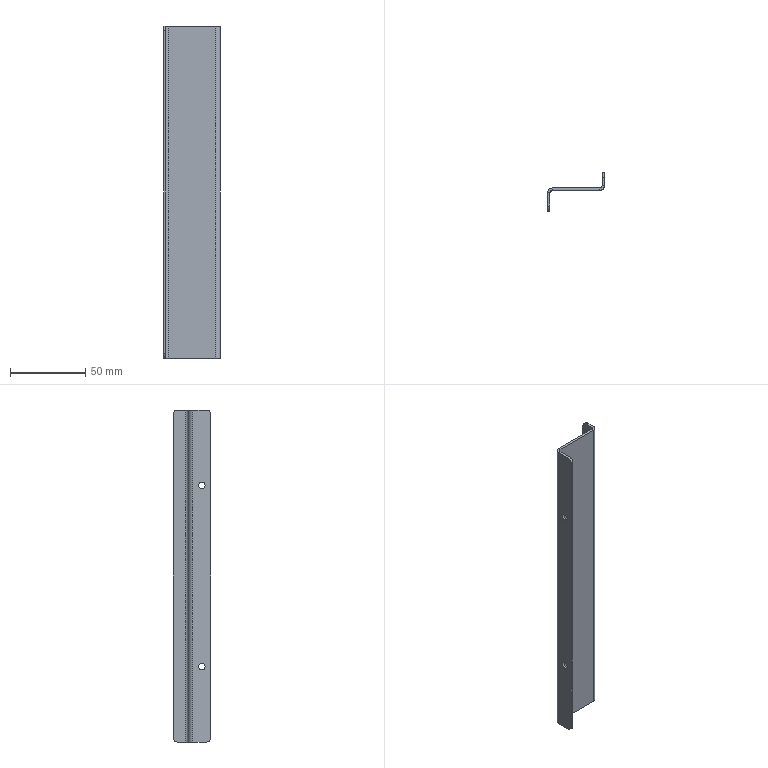Part | STEP file | 1 solid | 30 faces | box 37.5 x 25 x 220 mm | volume 19433 mm3 | plane 18 | cylinder 12 | commonest cylinder face diameters 6 x6 4.5 x4 3 x2